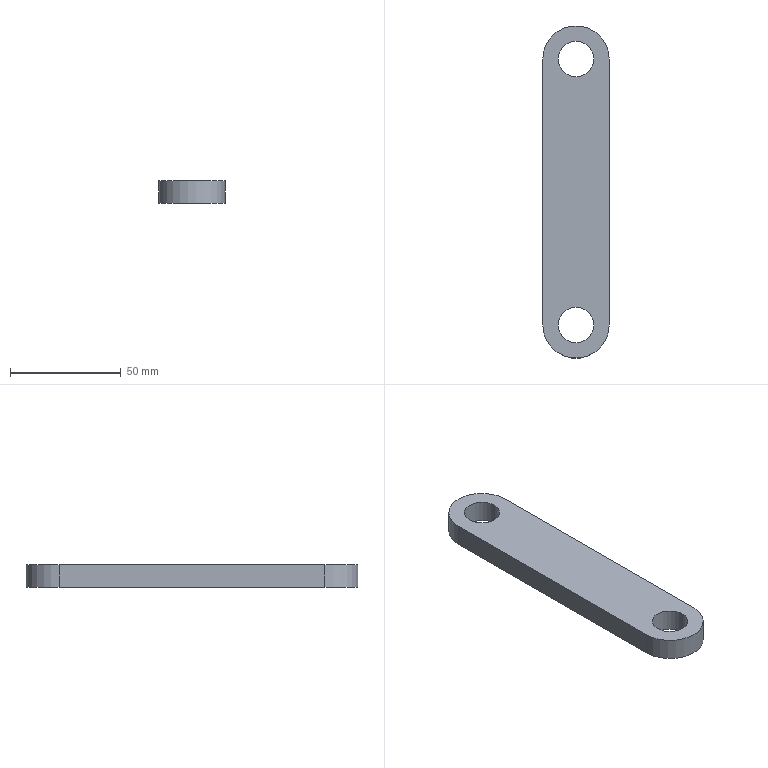Part | SolidWorks | features Extrusion 1 | 1 solid | 10 faces | box 30 x 150 x 10 mm | volume 39047 mm3 | cylinder 6 | plane 4 | commonest cylinder face diameters 16 x4 30 x2
STEP:
#1=CARTESIAN_POINT('',(-8.,-60.,10.));
#2=VERTEX_POINT('',#1);
#3=CARTESIAN_POINT('',(8.,-60.,10.));
#4=VERTEX_POINT('',#3);
#5=CARTESIAN_POINT('',(0.,-60.,10.));
#6=DIRECTION('',(0.,0.,1.));
#7=DIRECTION('',(1.,0.,0.));
#8=AXIS2_PLACEMENT_3D('',#5,#6,#7);
#9=CIRCLE('',#8,8.);
#10=EDGE_CURVE('',#2,#4,#9,.T.);
#11=ORIENTED_EDGE('',*,*,#10,.T.);
#12=CARTESIAN_POINT('',(8.,-60.,0.));
#13=VERTEX_POINT('',#12);
#14=CARTESIAN_POINT('',(8.,-60.,10.));
#15=DIRECTION('',(0.,0.,-1.));
#16=VECTOR('',#15,1000.);
#17=LINE('',#14,#16);
#18=EDGE_CURVE('',#4,#13,#17,.T.);
#19=ORIENTED_EDGE('',*,*,#18,.T.);
#20=CARTESIAN_POINT('',(-8.,-60.,0.));
#21=VERTEX_POINT('',#20);
#22=CARTESIAN_POINT('',(0.,-60.,0.));
#23=DIRECTION('',(0.,0.,1.));
#24=DIRECTION('',(1.,0.,0.));
#25=AXIS2_PLACEMENT_3D('',#22,#23,#24);
#26=CIRCLE('',#25,8.);
#27=EDGE_CURVE('',#21,#13,#26,.T.);
#28=ORIENTED_EDGE('',*,*,#27,.F.);
#29=CARTESIAN_POINT('',(-8.,-60.,10.));
#30=DIRECTION('',(0.,0.,-1.));
#31=VECTOR('',#30,1000.);
#32=LINE('',#29,#31);
#33=EDGE_CURVE('',#2,#21,#32,.T.);
#34=ORIENTED_EDGE('',*,*,#33,.F.);
#35=EDGE_LOOP('',(#11,#19,#28,#34));
#36=FACE_OUTER_BOUND('',#35,.T.);
#37=CARTESIAN_POINT('',(0.,-60.,10.));
#38=DIRECTION('',(0.,0.,-1.));
#39=DIRECTION('',(-1.,0.,0.));
#40=AXIS2_PLACEMENT_3D('',#37,#38,#39);
#41=CYLINDRICAL_SURFACE('',#40,8.);
#42=ADVANCED_FACE('',(#36),#41,.F.);
#43=CARTESIAN_POINT('',(-8.,60.,10.));
#44=VERTEX_POINT('',#43);
#45=CARTESIAN_POINT('',(8.,60.,10.));
#46=VERTEX_POINT('',#45);
#47=CARTESIAN_POINT('',(0.,60.,10.));
#48=DIRECTION('',(0.,0.,1.));
#49=DIRECTION('',(1.,0.,0.));
#50=AXIS2_PLACEMENT_3D('',#47,#48,#49);
#51=CIRCLE('',#50,8.);
#52=EDGE_CURVE('',#44,#46,#51,.T.);
#53=ORIENTED_EDGE('',*,*,#52,.T.);
#54=CARTESIAN_POINT('',(8.,60.,0.));
#55=VERTEX_POINT('',#54);
#56=CARTESIAN_POINT('',(8.,60.,10.));
#57=DIRECTION('',(0.,0.,-1.));
#58=VECTOR('',#57,1000.);
#59=LINE('',#56,#58);
#60=EDGE_CURVE('',#46,#55,#59,.T.);
#61=ORIENTED_EDGE('',*,*,#60,.T.);
#62=CARTESIAN_POINT('',(-8.,60.,0.));
#63=VERTEX_POINT('',#62);
#64=CARTESIAN_POINT('',(0.,60.,0.));
#65=DIRECTION('',(0.,0.,1.));
#66=DIRECTION('',(1.,0.,0.));
#67=AXIS2_PLACEMENT_3D('',#64,#65,#66);
#68=CIRCLE('',#67,8.);
#69=EDGE_CURVE('',#63,#55,#68,.T.);
#70=ORIENTED_EDGE('',*,*,#69,.F.);
#71=CARTESIAN_POINT('',(-8.,60.,10.));
#72=DIRECTION('',(0.,0.,-1.));
#73=VECTOR('',#72,1000.);
#74=LINE('',#71,#73);
#75=EDGE_CURVE('',#44,#63,#74,.T.);
#76=ORIENTED_EDGE('',*,*,#75,.F.);
#77=EDGE_LOOP('',(#53,#61,#70,#76));
#78=FACE_OUTER_BOUND('',#77,.T.);
#79=CARTESIAN_POINT('',(0.,60.,10.));
#80=DIRECTION('',(0.,0.,-1.));
#81=DIRECTION('',(-1.,0.,0.));
#82=AXIS2_PLACEMENT_3D('',#79,#80,#81);
#83=CYLINDRICAL_SURFACE('',#82,8.);
#84=ADVANCED_FACE('',(#78),#83,.F.);
#85=ORIENTED_EDGE('',*,*,#52,.F.);
#86=CARTESIAN_POINT('',(0.,60.,10.));
#87=DIRECTION('',(0.,0.,1.));
#88=DIRECTION('',(1.,0.,0.));
#89=AXIS2_PLACEMENT_3D('',#86,#87,#88);
#90=CIRCLE('',#89,8.);
#91=EDGE_CURVE('',#46,#44,#90,.T.);
#92=ORIENTED_EDGE('',*,*,#91,.F.);
#93=EDGE_LOOP('',(#85,#92));
#94=FACE_BOUND('',#93,.T.);
#95=CARTESIAN_POINT('',(-15.,-60.,10.));
#96=VERTEX_POINT('',#95);
#97=CARTESIAN_POINT('',(15.,-60.,10.));
#98=VERTEX_POINT('',#97);
#99=CARTESIAN_POINT('',(0.,-60.,10.));
#100=DIRECTION('',(0.,0.,1.));
#101=DIRECTION('',(1.,0.,0.));
#102=AXIS2_PLACEMENT_3D('',#99,#100,#101);
#103=CIRCLE('',#102,15.);
#104=EDGE_CURVE('',#96,#98,#103,.T.);
#105=ORIENTED_EDGE('',*,*,#104,.T.);
#106=CARTESIAN_POINT('',(15.,60.,10.));
#107=VERTEX_POINT('',#106);
#108=CARTESIAN_POINT('',(15.,60.,10.));
#109=DIRECTION('',(0.,1.,0.));
#110=VECTOR('',#109,1000.);
#111=LINE('',#108,#110);
#112=EDGE_CURVE('',#98,#107,#111,.T.);
#113=ORIENTED_EDGE('',*,*,#112,.T.);
#114=CARTESIAN_POINT('',(-15.,60.,10.));
#115=VERTEX_POINT('',#114);
#116=CARTESIAN_POINT('',(0.,60.,10.));
#117=DIRECTION('',(0.,0.,1.));
#118=DIRECTION('',(1.,0.,0.));
#119=AXIS2_PLACEMENT_3D('',#116,#117,#118);
#120=CIRCLE('',#119,15.);
#121=EDGE_CURVE('',#107,#115,#120,.T.);
#122=ORIENTED_EDGE('',*,*,#121,.T.);
#123=CARTESIAN_POINT('',(-15.,60.,10.));
#124=DIRECTION('',(0.,-1.,0.));
#125=VECTOR('',#124,1000.);
#126=LINE('',#123,#125);
#127=EDGE_CURVE('',#115,#96,#126,.T.);
#128=ORIENTED_EDGE('',*,*,#127,.T.);
#129=EDGE_LOOP('',(#105,#113,#122,#128));
#130=FACE_OUTER_BOUND('',#129,.T.);
#131=ORIENTED_EDGE('',*,*,#10,.F.);
#132=CARTESIAN_POINT('',(0.,-60.,10.));
#133=DIRECTION('',(0.,0.,1.));
#134=DIRECTION('',(1.,0.,0.));
#135=AXIS2_PLACEMENT_3D('',#132,#133,#134);
#136=CIRCLE('',#135,8.);
#137=EDGE_CURVE('',#4,#2,#136,.T.);
#138=ORIENTED_EDGE('',*,*,#137,.F.);
#139=EDGE_LOOP('',(#131,#138));
#140=FACE_BOUND('',#139,.T.);
#141=CARTESIAN_POINT('',(0.,-60.,10.));
#142=DIRECTION('',(0.,0.,1.));
#143=DIRECTION('',(1.,0.,0.));
#144=AXIS2_PLACEMENT_3D('',#141,#142,#143);
#145=PLANE('',#144);
#146=ADVANCED_FACE('',(#94,#130,#140),#145,.T.);
#147=CARTESIAN_POINT('',(-15.,-60.,0.));
#148=VERTEX_POINT('',#147);
#149=CARTESIAN_POINT('',(15.,-60.,0.));
#150=VERTEX_POINT('',#149);
#151=CARTESIAN_POINT('',(0.,-60.,0.));
#152=DIRECTION('',(0.,0.,1.));
#153=DIRECTION('',(1.,0.,0.));
#154=AXIS2_PLACEMENT_3D('',#151,#152,#153);
#155=CIRCLE('',#154,15.);
#156=EDGE_CURVE('',#148,#150,#155,.T.);
#157=ORIENTED_EDGE('',*,*,#156,.F.);
#158=CARTESIAN_POINT('',(-15.,60.,0.));
#159=VERTEX_POINT('',#158);
#160=CARTESIAN_POINT('',(-15.,60.,0.));
#161=DIRECTION('',(0.,-1.,0.));
#162=VECTOR('',#161,1000.);
#163=LINE('',#160,#162);
#164=EDGE_CURVE('',#159,#148,#163,.T.);
#165=ORIENTED_EDGE('',*,*,#164,.F.);
#166=CARTESIAN_POINT('',(15.,60.,0.));
#167=VERTEX_POINT('',#166);
#168=CARTESIAN_POINT('',(0.,60.,0.));
#169=DIRECTION('',(0.,0.,1.));
#170=DIRECTION('',(1.,0.,0.));
#171=AXIS2_PLACEMENT_3D('',#168,#169,#170);
#172=CIRCLE('',#171,15.);
#173=EDGE_CURVE('',#167,#159,#172,.T.);
#174=ORIENTED_EDGE('',*,*,#173,.F.);
#175=CARTESIAN_POINT('',(15.,60.,0.));
#176=DIRECTION('',(0.,1.,0.));
#177=VECTOR('',#176,1000.);
#178=LINE('',#175,#177);
#179=EDGE_CURVE('',#150,#167,#178,.T.);
#180=ORIENTED_EDGE('',*,*,#179,.F.);
#181=EDGE_LOOP('',(#157,#165,#174,#180));
#182=FACE_OUTER_BOUND('',#181,.T.);
#183=ORIENTED_EDGE('',*,*,#69,.T.);
#184=CARTESIAN_POINT('',(0.,60.,0.));
#185=DIRECTION('',(0.,0.,1.));
#186=DIRECTION('',(1.,0.,0.));
#187=AXIS2_PLACEMENT_3D('',#184,#185,#186);
#188=CIRCLE('',#187,8.);
#189=EDGE_CURVE('',#55,#63,#188,.T.);
#190=ORIENTED_EDGE('',*,*,#189,.T.);
#191=EDGE_LOOP('',(#183,#190));
#192=FACE_BOUND('',#191,.T.);
#193=ORIENTED_EDGE('',*,*,#27,.T.);
#194=CARTESIAN_POINT('',(0.,-60.,0.));
#195=DIRECTION('',(0.,0.,1.));
#196=DIRECTION('',(1.,0.,0.));
#197=AXIS2_PLACEMENT_3D('',#194,#195,#196);
#198=CIRCLE('',#197,8.);
#199=EDGE_CURVE('',#13,#21,#198,.T.);
#200=ORIENTED_EDGE('',*,*,#199,.T.);
#201=EDGE_LOOP('',(#193,#200));
#202=FACE_BOUND('',#201,.T.);
#203=CARTESIAN_POINT('',(0.,-60.,0.));
#204=DIRECTION('',(0.,0.,1.));
#205=DIRECTION('',(1.,0.,0.));
#206=AXIS2_PLACEMENT_3D('',#203,#204,#205);
#207=PLANE('',#206);
#208=ADVANCED_FACE('',(#182,#192,#202),#207,.F.);
#209=ORIENTED_EDGE('',*,*,#156,.T.);
#210=CARTESIAN_POINT('',(15.,-60.,10.));
#211=DIRECTION('',(0.,0.,-1.));
#212=VECTOR('',#211,1000.);
#213=LINE('',#210,#212);
#214=EDGE_CURVE('',#98,#150,#213,.T.);
#215=ORIENTED_EDGE('',*,*,#214,.F.);
#216=ORIENTED_EDGE('',*,*,#104,.F.);
#217=CARTESIAN_POINT('',(-15.,-60.,10.));
#218=DIRECTION('',(0.,0.,-1.));
#219=VECTOR('',#218,1000.);
#220=LINE('',#217,#219);
#221=EDGE_CURVE('',#96,#148,#220,.T.);
#222=ORIENTED_EDGE('',*,*,#221,.T.);
#223=EDGE_LOOP('',(#209,#215,#216,#222));
#224=FACE_OUTER_BOUND('',#223,.T.);
#225=CARTESIAN_POINT('',(0.,-60.,10.));
#226=DIRECTION('',(0.,0.,-1.));
#227=DIRECTION('',(-1.,0.,0.));
#228=AXIS2_PLACEMENT_3D('',#225,#226,#227);
#229=CYLINDRICAL_SURFACE('',#228,15.);
#230=ADVANCED_FACE('',(#224),#229,.T.);
#231=ORIENTED_EDGE('',*,*,#179,.T.);
#232=CARTESIAN_POINT('',(15.,60.,10.));
#233=DIRECTION('',(0.,0.,-1.));
#234=VECTOR('',#233,1000.);
#235=LINE('',#232,#234);
#236=EDGE_CURVE('',#107,#167,#235,.T.);
#237=ORIENTED_EDGE('',*,*,#236,.F.);
#238=ORIENTED_EDGE('',*,*,#112,.F.);
#239=ORIENTED_EDGE('',*,*,#214,.T.);
#240=EDGE_LOOP('',(#231,#237,#238,#239));
#241=FACE_OUTER_BOUND('',#240,.T.);
#242=CARTESIAN_POINT('',(15.,60.,10.));
#243=DIRECTION('',(-1.,0.,0.));
#244=DIRECTION('',(0.,-1.,0.));
#245=AXIS2_PLACEMENT_3D('',#242,#243,#244);
#246=PLANE('',#245);
#247=ADVANCED_FACE('',(#241),#246,.F.);
#248=ORIENTED_EDGE('',*,*,#173,.T.);
#249=CARTESIAN_POINT('',(-15.,60.,10.));
#250=DIRECTION('',(0.,0.,-1.));
#251=VECTOR('',#250,1000.);
#252=LINE('',#249,#251);
#253=EDGE_CURVE('',#115,#159,#252,.T.);
#254=ORIENTED_EDGE('',*,*,#253,.F.);
#255=ORIENTED_EDGE('',*,*,#121,.F.);
#256=ORIENTED_EDGE('',*,*,#236,.T.);
#257=EDGE_LOOP('',(#248,#254,#255,#256));
#258=FACE_OUTER_BOUND('',#257,.T.);
#259=CARTESIAN_POINT('',(0.,60.,10.));
#260=DIRECTION('',(0.,0.,-1.));
#261=DIRECTION('',(-1.,0.,0.));
#262=AXIS2_PLACEMENT_3D('',#259,#260,#261);
#263=CYLINDRICAL_SURFACE('',#262,15.);
#264=ADVANCED_FACE('',(#258),#263,.T.);
#265=ORIENTED_EDGE('',*,*,#164,.T.);
#266=ORIENTED_EDGE('',*,*,#221,.F.);
#267=ORIENTED_EDGE('',*,*,#127,.F.);
#268=ORIENTED_EDGE('',*,*,#253,.T.);
#269=EDGE_LOOP('',(#265,#266,#267,#268));
#270=FACE_OUTER_BOUND('',#269,.T.);
#271=CARTESIAN_POINT('',(-15.,60.,10.));
#272=DIRECTION('',(1.,0.,0.));
#273=DIRECTION('',(0.,1.,0.));
#274=AXIS2_PLACEMENT_3D('',#271,#272,#273);
#275=PLANE('',#274);
#276=ADVANCED_FACE('',(#270),#275,.F.);
#277=ORIENTED_EDGE('',*,*,#60,.F.);
#278=ORIENTED_EDGE('',*,*,#91,.T.);
#279=ORIENTED_EDGE('',*,*,#75,.T.);
#280=ORIENTED_EDGE('',*,*,#189,.F.);
#281=EDGE_LOOP('',(#277,#278,#279,#280));
#282=FACE_OUTER_BOUND('',#281,.T.);
#283=CARTESIAN_POINT('',(0.,60.,10.));
#284=DIRECTION('',(0.,0.,-1.));
#285=DIRECTION('',(-1.,0.,0.));
#286=AXIS2_PLACEMENT_3D('',#283,#284,#285);
#287=CYLINDRICAL_SURFACE('',#286,8.);
#288=ADVANCED_FACE('',(#282),#287,.F.);
#289=ORIENTED_EDGE('',*,*,#18,.F.);
#290=ORIENTED_EDGE('',*,*,#137,.T.);
#291=ORIENTED_EDGE('',*,*,#33,.T.);
#292=ORIENTED_EDGE('',*,*,#199,.F.);
#293=EDGE_LOOP('',(#289,#290,#291,#292));
#294=FACE_OUTER_BOUND('',#293,.T.);
#295=CARTESIAN_POINT('',(0.,-60.,10.));
#296=DIRECTION('',(0.,0.,-1.));
#297=DIRECTION('',(-1.,0.,0.));
#298=AXIS2_PLACEMENT_3D('',#295,#296,#297);
#299=CYLINDRICAL_SURFACE('',#298,8.);
#300=ADVANCED_FACE('',(#294),#299,.F.);
#301=CLOSED_SHELL('',(#42,#84,#146,#208,#230,#247,#264,#276,#288,#300));
#302=MANIFOLD_SOLID_BREP('',#301);
#303=CARTESIAN_POINT('',(0.,0.,0.));
#304=DIRECTION('',(0.,0.,1.));
#305=DIRECTION('',(1.,0.,0.));
#306=AXIS2_PLACEMENT_3D('',#303,#304,#305);
#307=(LENGTH_UNIT()NAMED_UNIT(*)SI_UNIT(.MILLI.,.METRE.));
#308=UNCERTAINTY_MEASURE_WITH_UNIT(LENGTH_MEASURE(0.00001),#307,'','');
#309=(NAMED_UNIT(*)PLANE_ANGLE_UNIT()SI_UNIT($,.RADIAN.));
#310=(NAMED_UNIT(*)SI_UNIT($,.STERADIAN.)SOLID_ANGLE_UNIT());
#311=(GEOMETRIC_REPRESENTATION_CONTEXT(3)GLOBAL_UNCERTAINTY_ASSIGNED_CONTEXT((#308))GLOBAL_UNIT_ASSIGNED_CONTEXT((#307,#309,#310))REPRESENTATION_CONTEXT('',''));
#312=ADVANCED_BREP_SHAPE_REPRESENTATION('',(#302,#306),#311);